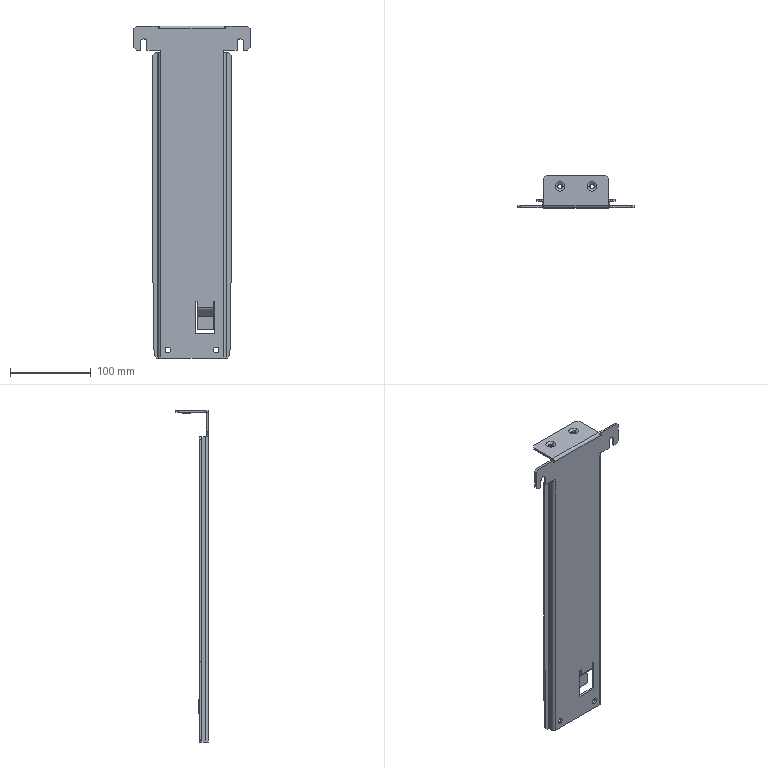Part | STEP file | 64728407 | 1 solid | 136 faces | box 144 x 40 x 412 mm | volume 121719 mm3 | plane 88 | cylinder 30 | torus 16 | spline 2 | commonest cylinder face diameters 1.6 x7 6.6 x7 5 x4 7 x4 10 x4 2 x2